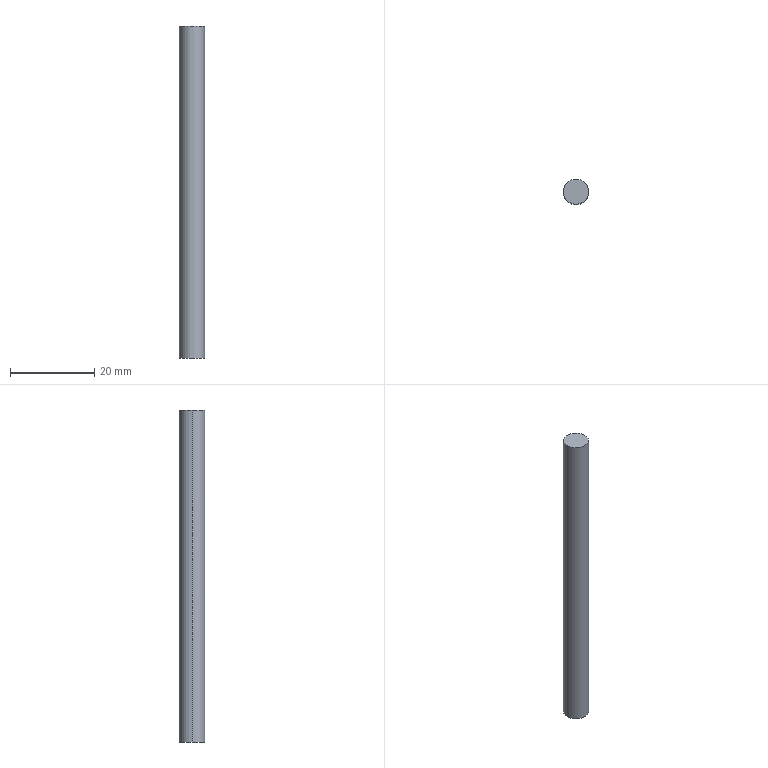Part | SolidWorks | features BaseBody 1 | 1 solid | 4 faces | box 6 x 6 x 79 mm | volume 2234 mm3 | cylinder 2 | plane 2 | commonest cylinder face diameters 6 x2
STEP:
#1=CARTESIAN_POINT('',(-20.,1556.,1039.));
#2=VERTEX_POINT('',#1);
#3=CARTESIAN_POINT('',(-26.,1556.,1039.));
#4=VERTEX_POINT('',#3);
#5=CARTESIAN_POINT('',(-23.,1556.,1039.));
#6=DIRECTION('',(0.,0.,1.));
#7=DIRECTION('',(1.,0.,0.));
#8=AXIS2_PLACEMENT_3D('',#5,#6,#7);
#9=CIRCLE('',#8,3.);
#10=EDGE_CURVE('',#2,#4,#9,.T.);
#11=ORIENTED_EDGE('',*,*,#10,.T.);
#12=CARTESIAN_POINT('',(-26.,1556.,1118.));
#13=VERTEX_POINT('',#12);
#14=CARTESIAN_POINT('',(-26.,1556.,1039.));
#15=DIRECTION('',(0.,0.,1.));
#16=VECTOR('',#15,1000.);
#17=LINE('',#14,#16);
#18=EDGE_CURVE('',#4,#13,#17,.T.);
#19=ORIENTED_EDGE('',*,*,#18,.T.);
#20=CARTESIAN_POINT('',(-20.,1556.,1118.));
#21=VERTEX_POINT('',#20);
#22=CARTESIAN_POINT('',(-23.,1556.,1118.));
#23=DIRECTION('',(0.,0.,1.));
#24=DIRECTION('',(1.,0.,0.));
#25=AXIS2_PLACEMENT_3D('',#22,#23,#24);
#26=CIRCLE('',#25,3.);
#27=EDGE_CURVE('',#21,#13,#26,.T.);
#28=ORIENTED_EDGE('',*,*,#27,.F.);
#29=CARTESIAN_POINT('',(-20.,1556.,1039.));
#30=DIRECTION('',(0.,0.,1.));
#31=VECTOR('',#30,1000.);
#32=LINE('',#29,#31);
#33=EDGE_CURVE('',#2,#21,#32,.T.);
#34=ORIENTED_EDGE('',*,*,#33,.F.);
#35=EDGE_LOOP('',(#11,#19,#28,#34));
#36=FACE_OUTER_BOUND('',#35,.T.);
#37=CARTESIAN_POINT('',(-23.,1556.,1039.));
#38=DIRECTION('',(0.,0.,1.));
#39=DIRECTION('',(1.,0.,0.));
#40=AXIS2_PLACEMENT_3D('',#37,#38,#39);
#41=CYLINDRICAL_SURFACE('',#40,3.);
#42=ADVANCED_FACE('',(#36),#41,.T.);
#43=ORIENTED_EDGE('',*,*,#10,.F.);
#44=CARTESIAN_POINT('',(-23.,1556.,1039.));
#45=DIRECTION('',(0.,0.,1.));
#46=DIRECTION('',(1.,0.,0.));
#47=AXIS2_PLACEMENT_3D('',#44,#45,#46);
#48=CIRCLE('',#47,3.);
#49=EDGE_CURVE('',#4,#2,#48,.T.);
#50=ORIENTED_EDGE('',*,*,#49,.F.);
#51=EDGE_LOOP('',(#43,#50));
#52=FACE_OUTER_BOUND('',#51,.T.);
#53=CARTESIAN_POINT('',(-26.12,1552.88,1039.));
#54=DIRECTION('',(0.,0.,1.));
#55=DIRECTION('',(1.,0.,0.));
#56=AXIS2_PLACEMENT_3D('',#53,#54,#55);
#57=PLANE('',#56);
#58=ADVANCED_FACE('',(#52),#57,.F.);
#59=ORIENTED_EDGE('',*,*,#18,.F.);
#60=ORIENTED_EDGE('',*,*,#49,.T.);
#61=ORIENTED_EDGE('',*,*,#33,.T.);
#62=CARTESIAN_POINT('',(-23.,1556.,1118.));
#63=DIRECTION('',(0.,0.,1.));
#64=DIRECTION('',(1.,0.,0.));
#65=AXIS2_PLACEMENT_3D('',#62,#63,#64);
#66=CIRCLE('',#65,3.);
#67=EDGE_CURVE('',#13,#21,#66,.T.);
#68=ORIENTED_EDGE('',*,*,#67,.F.);
#69=EDGE_LOOP('',(#59,#60,#61,#68));
#70=FACE_OUTER_BOUND('',#69,.T.);
#71=CARTESIAN_POINT('',(-23.,1556.,1039.));
#72=DIRECTION('',(0.,0.,1.));
#73=DIRECTION('',(1.,0.,0.));
#74=AXIS2_PLACEMENT_3D('',#71,#72,#73);
#75=CYLINDRICAL_SURFACE('',#74,3.);
#76=ADVANCED_FACE('',(#70),#75,.T.);
#77=ORIENTED_EDGE('',*,*,#27,.T.);
#78=ORIENTED_EDGE('',*,*,#67,.T.);
#79=EDGE_LOOP('',(#77,#78));
#80=FACE_OUTER_BOUND('',#79,.T.);
#81=CARTESIAN_POINT('',(-26.12,1552.88,1118.));
#82=DIRECTION('',(0.,0.,1.));
#83=DIRECTION('',(1.,0.,0.));
#84=AXIS2_PLACEMENT_3D('',#81,#82,#83);
#85=PLANE('',#84);
#86=ADVANCED_FACE('',(#80),#85,.T.);
#87=CLOSED_SHELL('',(#42,#58,#76,#86));
#88=MANIFOLD_SOLID_BREP('',#87);
#89=CARTESIAN_POINT('',(0.,0.,0.));
#90=DIRECTION('',(0.,0.,1.));
#91=DIRECTION('',(1.,0.,0.));
#92=AXIS2_PLACEMENT_3D('',#89,#90,#91);
#93=(LENGTH_UNIT()NAMED_UNIT(*)SI_UNIT(.MILLI.,.METRE.));
#94=UNCERTAINTY_MEASURE_WITH_UNIT(LENGTH_MEASURE(0.00001),#93,'','');
#95=(NAMED_UNIT(*)PLANE_ANGLE_UNIT()SI_UNIT($,.RADIAN.));
#96=(NAMED_UNIT(*)SI_UNIT($,.STERADIAN.)SOLID_ANGLE_UNIT());
#97=(GEOMETRIC_REPRESENTATION_CONTEXT(3)GLOBAL_UNCERTAINTY_ASSIGNED_CONTEXT((#94))GLOBAL_UNIT_ASSIGNED_CONTEXT((#93,#95,#96))REPRESENTATION_CONTEXT('',''));
#98=ADVANCED_BREP_SHAPE_REPRESENTATION('',(#88,#92),#97);